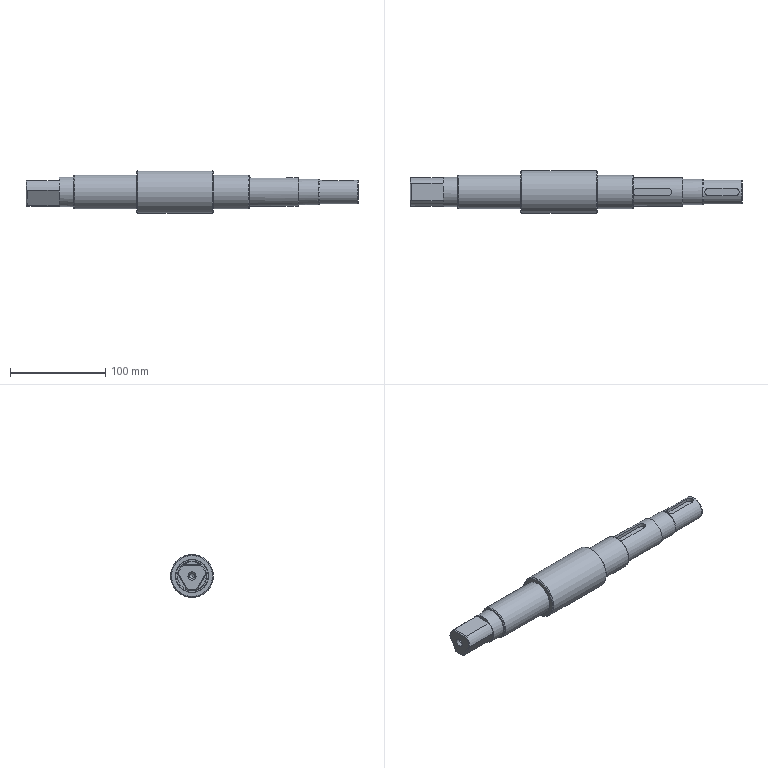NC program | NX | posted with a generic post | part box 348.4 x 45 x 45 mm
Lines 7257 to 8230 of 8230:
(PLANAR_MILL_COPY_COPY , TOOL : D6A45)
N14500 T07 M6
N14502 G54
N14504 G17 G0 G90 X13.51 Y-6.915 B0. C0. S7500 M3
N14506 G43 Z30. H7
N14508 Z0.5
N14510 G94 G1 Z-2.5 F1250.
N14512 G3 X12.818 Y-7.4 R1.
N14514 G1 X8.248 Y-15.315
N14516 G2 X6.473 Y-16.832 R3.5
N14518 X-6.473 Y-16.832 R18.034
N14520 X-8.248 Y-15.315 R3.5
N14522 G1 X-17.387 Y0.515
N14524 G2 X-17.813 Y2.81 R3.5
N14526 X-11.34 Y14.022 R18.034
N14528 X-9.139 Y14.801 R3.5
N14530 G1 X9.139
N14532 G2 X11.34 Y14.022 R3.5
N14534 X17.813 Y2.81 R18.034
N14536 X17.387 Y0.515 R3.5
N14538 G1 X12.818 Y-7.4
N14540 X12.385 Y-7.15
N14542 X7.815 Y-15.065
N14544 G2 X6.294 Y-16.365 R3.
N14546 X-6.294 Y-16.365 R17.534
N14548 X-7.815 Y-15.065 R3.
N14550 G1 X-16.954 Y0.765
N14552 G2 X-17.32 Y2.732 R3.
N14554 X-11.026 Y13.633 R17.534
N14556 X-9.139 Y14.301 R3.
N14558 G1 X9.139
N14560 G2 X11.026 Y13.633 R3.
N14562 X17.32 Y2.732 R17.534
N14564 X16.954 Y0.765 R3.
N14566 G1 X12.385 Y-7.15
N14568 X11.952 Y-6.9
N14570 X7.382 Y-14.815
N14572 G2 X6.114 Y-15.898 R2.5
N14574 X-6.114 Y-15.898 R17.034
N14576 X-7.382 Y-14.815 R2.5
N14578 G1 X-16.521 Y1.015
N14580 G2 X-16.826 Y2.654 R2.5
N14582 X-10.711 Y13.244 R17.034
N14584 X-9.139 Y13.801 R2.5
N14586 G1 X9.139
N14588 G2 X10.711 Y13.244 R2.5
N14590 X16.826 Y2.654 R17.034
N14592 X16.521 Y1.015 R2.5
N14594 G1 X11.952 Y-6.9
N14596 G3 X11.878 Y-7.742 R1.
N14598 G1 Z0.5
N14600 G0 Z30.
(PLANAR_MILL_COPY_COPY_COPY , TOOL : D6A45)
N14602 X0.766 Y1.143
N14604 Z1.5
N14606 G1 Z-1.5
N14608 G3 X0. Y1.5 R1.
N14610 X-1.5 Y0. R1.5
N14612 X0. Y1.5 R-1.5
N14614 X-0.766 Y1.143 R1.
N14616 G1 Z1.5
N14618 G0 Z30.
N14620 M5
(刀补12 , TOOL : D12)
N14622 T12 M6
N14624 G54
N14626 G17 G0 G90 X-12.039 Y-19.737 B0. C0. S5000 M3
N14628 G43 Z30. H12
N14630 Z1.
N14632 G94 G1 Z-1. F1250.
N14634 G41 X-11.975 Y-19.66 D12
N14636 X-11.079 Y-18.11
N14638 G3 X-11.079 Y-16.91 R1.2
N14640 G1 X-20.131 Y-1.232
N14642 G2 X-20.488 Y-0.507 R5.249
N14644 X-20.765 Y0.339 R6.776
N14646 X-20.863 Y2.801 R6.317
N14648 X-13.595 Y16.071 R21.05
N14650 X-12.592 Y16.868 R21.528
N14652 X-9.101 Y18.05 R6.061
N14654 G1 X-9.
N14656 X8.993
N14658 G2 X9.818 Y17.994 R5.44
N14660 X12.63 Y16.84 R6.029
N14662 X13.607 Y16.061 R21.048
N14664 X20.9 Y2.505 R21.
N14666 X20.133 Y-1.228 R6.039
N14668 G1 X11.132 Y-16.819
N14670 G2 X10.673 Y-17.502 R5.208
N14672 X8.257 Y-19.363 R6.188
N14674 X-8.171 Y-19.399 R21.05
N14676 X-11.079 Y-16.91 R6.067
N14678 G3 X-12.129 Y-16.329 R1.2
N14680 G1 X-14.165 Y-16.366
N14682 G40
N14684 X-14.263 Y-16.385
N14686 Z1.
N14688 G0 Z30.
N14690 X-12.002 Y-19.775
N14692 Z0.
N14694 G1 Z-2.
N14696 G41 X-11.939 Y-19.697
N14698 X-11.058 Y-18.109
N14700 G3 X-11.079 Y-16.909 R1.2
N14702 G1 X-11.132 Y-16.819
N14704 X-20.14 Y-1.217
N14706 G2 X-20.899 Y2.518 R6.05
N14708 X-12.63 Y16.84 R21.05
N14710 X-8.99 Y18.05 R6.05
N14712 G1 X9.
N14714 G2 X12.63 Y16.84 R6.05
N14716 X20.899 Y2.518 R21.05
N14718 X20.125 Y-1.243 R6.05
N14720 G1 X11.156 Y-16.777
N14722 X11.132 Y-16.82
N14724 G2 X8.269 Y-19.358 R6.05
N14726 X-8.269 Y-19.358 R21.05
N14728 X-11.079 Y-16.909 R6.05
N14730 G3 X-12.128 Y-16.327 R1.2
N14732 G1 X-14.167 Y-16.363
N14734 G40
N14736 X-14.265 Y-16.382
N14738 Z0.
N14740 G0 Z30.
N14742 X-12.002 Y-19.775
N14744 Z-1.
N14746 G1 Z-3.
N14748 G41 X-11.939 Y-19.697
N14750 X-11.058 Y-18.109
N14752 G3 X-11.079 Y-16.909 R1.2
N14754 G1 X-11.132 Y-16.819
N14756 X-20.14 Y-1.217
N14758 G2 X-20.899 Y2.518 R6.05
N14760 X-12.63 Y16.84 R21.05
N14762 X-8.99 Y18.05 R6.05
N14764 G1 X9.
N14766 G2 X12.63 Y16.84 R6.05
N14768 X20.899 Y2.518 R21.05
N14770 X20.125 Y-1.243 R6.05
N14772 G1 X11.156 Y-16.777
N14774 X11.131 Y-16.82
N14776 G2 X8.269 Y-19.358 R6.05
N14778 X-8.269 Y-19.358 R21.05
N14780 X-11.079 Y-16.909 R6.05
N14782 G3 X-12.128 Y-16.327 R1.2
N14784 G1 X-14.167 Y-16.363
N14786 G40
N14788 X-14.265 Y-16.382
N14790 Z-1.
N14792 G0 Z30.
N14794 X-12.002 Y-19.775
N14796 Z-2.
N14798 G1 Z-4.
N14800 G41 X-11.939 Y-19.697
N14802 X-11.058 Y-18.109
N14804 G3 X-11.079 Y-16.909 R1.2
N14806 G1 X-11.132 Y-16.819
N14808 X-20.14 Y-1.217
N14810 G2 X-20.899 Y2.518 R6.05
N14812 X-12.63 Y16.84 R21.05
N14814 X-8.99 Y18.05 R6.05
N14816 G1 X9.
N14818 G2 X12.63 Y16.84 R6.05
N14820 X20.899 Y2.518 R21.05
N14822 X20.125 Y-1.243 R6.05
N14824 G1 X11.156 Y-16.777
N14826 X11.131 Y-16.82
N14828 G2 X8.269 Y-19.358 R6.05
N14830 X-8.269 Y-19.358 R21.05
N14832 X-11.079 Y-16.909 R6.05
N14834 G3 X-12.128 Y-16.327 R1.2
N14836 G1 X-14.167 Y-16.363
N14838 G40
N14840 X-14.265 Y-16.382
N14842 Z-2.
N14844 G0 Z30.
N14846 X-12.002 Y-19.775
N14848 Z-3.
N14850 G1 Z-5.
N14852 G41 X-11.939 Y-19.697
N14854 X-11.058 Y-18.109
N14856 G3 X-11.079 Y-16.909 R1.2
N14858 G1 X-11.132 Y-16.819
N14860 X-20.14 Y-1.217
N14862 G2 X-20.899 Y2.518 R6.05
N14864 X-12.63 Y16.84 R21.05
N14866 X-8.99 Y18.05 R6.05
N14868 G1 X9.
N14870 G2 X12.63 Y16.84 R6.05
N14872 X20.899 Y2.518 R21.05
N14874 X20.125 Y-1.243 R6.05
N14876 G1 X11.156 Y-16.777
N14878 X11.131 Y-16.82
N14880 G2 X8.269 Y-19.358 R6.05
N14882 X-8.269 Y-19.358 R21.05
N14884 X-11.079 Y-16.909 R6.05
N14886 G3 X-12.128 Y-16.327 R1.2
N14888 G1 X-14.167 Y-16.363
N14890 G40
N14892 X-14.265 Y-16.382
N14894 Z-3.
N14896 G0 Z30.
N14898 X-12.002 Y-19.775
N14900 Z-4.
N14902 G1 Z-6.
N14904 G41 X-11.939 Y-19.697
N14906 X-11.058 Y-18.109
N14908 G3 X-11.079 Y-16.909 R1.2
N14910 G1 X-11.132 Y-16.819
N14912 X-20.14 Y-1.217
N14914 G2 X-20.899 Y2.518 R6.05
N14916 X-12.63 Y16.84 R21.05
N14918 X-8.99 Y18.05 R6.05
N14920 G1 X9.
N14922 G2 X12.63 Y16.84 R6.05
N14924 X20.899 Y2.518 R21.05
N14926 X20.125 Y-1.243 R6.05
N14928 G1 X11.156 Y-16.777
N14930 X11.131 Y-16.821
N14932 G2 X8.269 Y-19.358 R6.05
N14934 X-8.269 Y-19.358 R21.05
N14936 X-11.079 Y-16.909 R6.05
N14938 G3 X-12.128 Y-16.327 R1.2
N14940 G1 X-14.167 Y-16.363
N14942 G40
N14944 X-14.265 Y-16.382
N14946 Z-4.
N14948 G0 Z30.
N14950 X-12.002 Y-19.775
N14952 Z-5.
N14954 G1 Z-7.
N14956 G41 X-11.939 Y-19.697
N14958 X-11.058 Y-18.109
N14960 G3 X-11.079 Y-16.909 R1.2
N14962 G1 X-11.132 Y-16.819
N14964 X-20.14 Y-1.217
N14966 G2 X-20.899 Y2.518 R6.05
N14968 X-12.63 Y16.84 R21.05
N14970 X-8.99 Y18.05 R6.05
N14972 G1 X9.
N14974 G2 X12.63 Y16.84 R6.05
N14976 X20.899 Y2.518 R21.05
N14978 X20.125 Y-1.243 R6.05
N14980 G1 X11.156 Y-16.777
N14982 X11.131 Y-16.821
N14984 G2 X8.269 Y-19.358 R6.05
N14986 X-8.269 Y-19.358 R21.05
N14988 X-11.079 Y-16.909 R6.05
N14990 G3 X-12.128 Y-16.327 R1.2
N14992 G1 X-14.167 Y-16.363
N14994 G40
N14996 X-14.265 Y-16.382
N14998 Z-5.
N15000 G0 Z30.
N15002 X-12.002 Y-19.775
N15004 Z-6.
N15006 G1 Z-8.
N15008 G41 X-11.939 Y-19.697
N15010 X-11.058 Y-18.109
N15012 G3 X-11.079 Y-16.909 R1.2
N15014 G1 X-11.132 Y-16.819
N15016 X-20.132 Y-1.231
N15018 G2 X-20.899 Y2.518 R6.05
N15020 X-12.63 Y16.84 R21.05
N15022 X-8.99 Y18.05 R6.05
N15024 G1 X9.
N15026 G2 X12.63 Y16.84 R6.05
N15028 X20.899 Y2.518 R21.05
N15030 X20.125 Y-1.243 R6.05
N15032 G1 X11.156 Y-16.777
N15034 X11.131 Y-16.821
N15036 G2 X8.269 Y-19.358 R6.05
N15038 X-8.269 Y-19.358 R21.05
N15040 X-11.079 Y-16.909 R6.05
N15042 G3 X-12.128 Y-16.327 R1.2
N15044 G1 X-14.167 Y-16.363
N15046 G40
N15048 X-14.265 Y-16.382
N15050 Z-6.
N15052 G0 Z30.
N15054 X-12.002 Y-19.775
N15056 Z-7.
N15058 G1 Z-9.
N15060 G41 X-11.939 Y-19.697
N15062 X-11.058 Y-18.109
N15064 G3 X-11.079 Y-16.909 R1.2
N15066 G1 X-11.132 Y-16.819
N15068 X-20.132 Y-1.231
N15070 G2 X-20.899 Y2.518 R6.05
N15072 X-12.63 Y16.84 R21.05
N15074 X-8.99 Y18.05 R6.05
N15076 G1 X9.
N15078 G2 X12.63 Y16.84 R6.05
N15080 X20.899 Y2.518 R21.05
N15082 X20.125 Y-1.243 R6.05
N15084 G1 X11.156 Y-16.777
N15086 X11.13 Y-16.822
N15088 G2 X8.269 Y-19.358 R6.05
N15090 X-8.269 Y-19.358 R21.05
N15092 X-11.079 Y-16.909 R6.05
N15094 G3 X-12.128 Y-16.327 R1.2
N15096 G1 X-14.167 Y-16.363
N15098 G40
N15100 X-14.265 Y-16.382
N15102 Z-7.
N15104 G0 Z30.
N15106 X-12.002 Y-19.775
N15108 Z-8.
N15110 G1 Z-10.
N15112 G41 X-11.939 Y-19.697
N15114 X-11.058 Y-18.109
N15116 G3 X-11.079 Y-16.909 R1.2
N15118 G1 X-11.132 Y-16.819
N15120 X-20.132 Y-1.231
N15122 G2 X-20.899 Y2.518 R6.05
N15124 X-12.63 Y16.84 R21.05
N15126 X-8.99 Y18.05 R6.05
N15128 G1 X9.
N15130 G2 X12.63 Y16.84 R6.05
N15132 X20.899 Y2.518 R21.05
N15134 X20.125 Y-1.243 R6.05
N15136 G1 X11.156 Y-16.777
N15138 X11.13 Y-16.822
N15140 G2 X8.269 Y-19.358 R6.05
N15142 X-8.269 Y-19.358 R21.05
N15144 X-11.079 Y-16.909 R6.05
N15146 G3 X-12.128 Y-16.327 R1.2
N15148 G1 X-14.167 Y-16.363
N15150 G40
N15152 X-14.265 Y-16.382
N15154 Z-8.
N15156 G0 Z30.
N15158 X-12.002 Y-19.775
N15160 Z-9.
N15162 G1 Z-11.
N15164 G41 X-11.939 Y-19.697
N15166 X-11.058 Y-18.109
N15168 G3 X-11.079 Y-16.909 R1.2
N15170 G1 X-11.132 Y-16.819
N15172 X-20.132 Y-1.23
N15174 G2 X-20.899 Y2.518 R6.05
N15176 X-12.63 Y16.84 R21.05
N15178 X-8.99 Y18.05 R6.05
N15180 G1 X9.
N15182 G2 X12.63 Y16.84 R6.05
N15184 X20.899 Y2.518 R21.05
N15186 X20.125 Y-1.243 R6.05
N15188 G1 X11.156 Y-16.777
N15190 X11.13 Y-16.822
N15192 G2 X8.269 Y-19.358 R6.05
N15194 X-8.269 Y-19.358 R21.05
N15196 X-11.079 Y-16.909 R6.05
N15198 G3 X-12.128 Y-16.327 R1.2
N15200 G1 X-14.167 Y-16.363
N15202 G40
N15204 X-14.265 Y-16.382
N15206 Z-9.
N15208 G0 Z30.
N15210 X-12.002 Y-19.775
N15212 Z-10.
N15214 G1 Z-12.
N15216 G41 X-11.939 Y-19.697
N15218 X-11.058 Y-18.109
N15220 G3 X-11.079 Y-16.909 R1.2
N15222 G1 X-11.132 Y-16.819
N15224 X-20.132 Y-1.23
N15226 G2 X-20.899 Y2.518 R6.05
N15228 X-12.63 Y16.84 R21.05
N15230 X-8.99 Y18.05 R6.05
N15232 G1 X9.
N15234 G2 X12.63 Y16.84 R6.05
N15236 X20.899 Y2.518 R21.05
N15238 X20.125 Y-1.243 R6.05
N15240 G1 X11.156 Y-16.777
N15242 X11.13 Y-16.823
N15244 G2 X8.269 Y-19.358 R6.05
N15246 X-8.269 Y-19.358 R21.05
N15248 X-11.079 Y-16.909 R6.05
N15250 G3 X-12.128 Y-16.327 R1.2
N15252 G1 X-14.167 Y-16.363
N15254 G40
N15256 X-14.265 Y-16.382
N15258 Z-10.
N15260 G0 Z30.
N15262 X-12.002 Y-19.775
N15264 Z-11.
N15266 G1 Z-13.
N15268 G41 X-11.939 Y-19.697
N15270 X-11.058 Y-18.109
N15272 G3 X-11.079 Y-16.909 R1.2
N15274 G1 X-11.132 Y-16.819
N15276 X-20.132 Y-1.23
N15278 G2 X-20.899 Y2.518 R6.05
N15280 X-12.63 Y16.84 R21.05
N15282 X-8.99 Y18.05 R6.05
N15284 G1 X9.
N15286 G2 X12.63 Y16.84 R6.05
N15288 X20.899 Y2.518 R21.05
N15290 X20.125 Y-1.243 R6.05
N15292 G1 X11.156 Y-16.777
N15294 X11.129 Y-16.823
N15296 G2 X8.269 Y-19.358 R6.05
N15298 X-8.269 Y-19.358 R21.05
N15300 X-11.079 Y-16.909 R6.05
N15302 G3 X-12.128 Y-16.327 R1.2
N15304 G1 X-14.167 Y-16.363
N15306 G40
N15308 X-14.265 Y-16.382
N15310 Z-11.
N15312 G0 Z30.
N15314 X-12.002 Y-19.775
N15316 Z-12.
N15318 G1 Z-14.
N15320 G41 X-11.939 Y-19.697
N15322 X-11.058 Y-18.109
N15324 G3 X-11.079 Y-16.909 R1.2
N15326 G1 X-11.132 Y-16.819
N15328 X-20.133 Y-1.229
N15330 G2 X-20.899 Y2.518 R6.05
N15332 X-12.63 Y16.84 R21.05
N15334 X-8.99 Y18.05 R6.05
N15336 G1 X9.
N15338 G2 X12.63 Y16.84 R6.05
N15340 X20.899 Y2.518 R21.05
N15342 X20.125 Y-1.243 R6.05
N15344 G1 X11.156 Y-16.777
N15346 X11.129 Y-16.824
N15348 G2 X8.269 Y-19.358 R6.05
N15350 X-8.269 Y-19.358 R21.05
N15352 X-11.079 Y-16.909 R6.05
N15354 G3 X-12.128 Y-16.327 R1.2
N15356 G1 X-14.167 Y-16.363
N15358 G40
N15360 X-14.265 Y-16.382
N15362 Z-12.
N15364 G0 Z30.
N15366 X-12.002 Y-19.775
N15368 Z-13.
N15370 G1 Z-15.
N15372 G41 X-11.939 Y-19.697
N15374 X-11.058 Y-18.109
N15376 G3 X-11.079 Y-16.909 R1.2
N15378 G1 X-11.132 Y-16.819
N15380 X-20.133 Y-1.229
N15382 G2 X-20.899 Y2.518 R6.05
N15384 X-12.63 Y16.84 R21.05
N15386 X-8.99 Y18.05 R6.05
N15388 G1 X9.
N15390 G2 X12.63 Y16.84 R6.05
N15392 X20.899 Y2.518 R21.05
N15394 X20.125 Y-1.243 R6.05
N15396 G1 X11.156 Y-16.777
N15398 X11.129 Y-16.824
N15400 G2 X8.269 Y-19.358 R6.05
N15402 X-8.269 Y-19.358 R21.05
N15404 X-11.079 Y-16.909 R6.05
N15406 G3 X-12.128 Y-16.327 R1.2
N15408 G1 X-14.167 Y-16.363
N15410 G40
N15412 X-14.265 Y-16.382
N15414 Z-13.
N15416 G0 Z30.
N15418 X-12.002 Y-19.775
N15420 Z-14.
N15422 G1 Z-16.
N15424 G41 X-11.939 Y-19.697
N15426 X-11.058 Y-18.109
N15428 G3 X-11.079 Y-16.909 R1.2
N15430 G1 X-11.132 Y-16.819
N15432 X-20.133 Y-1.229
N15434 G2 X-20.899 Y2.518 R6.05
N15436 X-12.63 Y16.84 R21.05
N15438 X-8.99 Y18.05 R6.05
N15440 G1 X9.
N15442 G2 X12.63 Y16.84 R6.05
N15444 X20.899 Y2.518 R21.05
N15446 X20.125 Y-1.243 R6.05
N15448 G1 X11.156 Y-16.777
N15450 X11.129 Y-16.825
N15452 G2 X8.269 Y-19.358 R6.05
N15454 X-8.269 Y-19.358 R21.05
N15456 X-11.079 Y-16.909 R6.05
N15458 G3 X-12.128 Y-16.327 R1.2
N15460 G1 X-14.167 Y-16.363
N15462 G40
N15464 X-14.265 Y-16.382
N15466 Z-14.
N15468 G0 Z30.
N15470 X-12.002 Y-19.775
N15472 Z-15.
N15474 G1 Z-17.
N15476 G41 X-11.939 Y-19.697
N15478 X-11.058 Y-18.109
N15480 G3 X-11.079 Y-16.909 R1.2
N15482 G1 X-11.132 Y-16.819
N15484 X-20.133 Y-1.228
N15486 G2 X-20.899 Y2.518 R6.05
N15488 X-12.63 Y16.84 R21.05
N15490 X-8.99 Y18.05 R6.05
N15492 G1 X9.
N15494 G2 X12.63 Y16.84 R6.05
N15496 X20.899 Y2.518 R21.05
N15498 X20.125 Y-1.243 R6.05
N15500 G1 X11.156 Y-16.777
N15502 X11.128 Y-16.825
N15504 G2 X8.269 Y-19.358 R6.05
N15506 X-8.269 Y-19.358 R21.05
N15508 X-11.079 Y-16.909 R6.05
N15510 G3 X-12.128 Y-16.327 R1.2
N15512 G1 X-14.167 Y-16.363
N15514 G40
N15516 X-14.265 Y-16.382
N15518 Z-15.
N15520 G0 Z30.
N15522 X-12.002 Y-19.775
N15524 Z-16.
N15526 G1 Z-18.
N15528 G41 X-11.939 Y-19.697
N15530 X-11.058 Y-18.109
N15532 G3 X-11.079 Y-16.909 R1.2
N15534 G1 X-11.132 Y-16.819
N15536 X-20.134 Y-1.227
N15538 G2 X-20.899 Y2.518 R6.05
N15540 X-12.63 Y16.84 R21.05
N15542 X-8.99 Y18.05 R6.05
N15544 G1 X9.
N15546 G2 X12.63 Y16.84 R6.05
N15548 X20.899 Y2.518 R21.05
N15550 X20.125 Y-1.243 R6.05
N15552 G1 X11.156 Y-16.777
N15554 X11.128 Y-16.826
N15556 G2 X8.269 Y-19.358 R6.05
N15558 X-8.269 Y-19.358 R21.05
N15560 X-11.079 Y-16.909 R6.05
N15562 G3 X-12.128 Y-16.327 R1.2
N15564 G1 X-14.167 Y-16.363
N15566 G40
N15568 X-14.265 Y-16.382
N15570 Z-16.
N15572 G0 Z30.
N15574 X-12.002 Y-19.775
N15576 Z-17.
N15578 G1 Z-19.
N15580 G41 X-11.939 Y-19.697
N15582 X-11.058 Y-18.109
N15584 G3 X-11.079 Y-16.909 R1.2
N15586 G1 X-11.132 Y-16.819
N15588 X-20.134 Y-1.227
N15590 G2 X-20.899 Y2.518 R6.05
N15592 X-12.63 Y16.84 R21.05
N15594 X-8.99 Y18.05 R6.05
N15596 G1 X9.
N15598 G2 X12.63 Y16.84 R6.05
N15600 X20.899 Y2.518 R21.05
N15602 X20.132 Y-1.231 R6.05
N15604 G1 X11.156 Y-16.777
N15606 X11.127 Y-16.827
N15608 G2 X8.269 Y-19.358 R6.05
N15610 X-8.269 Y-19.358 R21.05
N15612 X-11.079 Y-16.909 R6.05
N15614 G3 X-12.128 Y-16.327 R1.2
N15616 G1 X-14.167 Y-16.363
N15618 G40
N15620 X-14.265 Y-16.382
N15622 Z-17.
N15624 G0 Z30.
N15626 X-12.002 Y-19.775
N15628 Z-18.
N15630 G1 Z-20.
N15632 G41 X-11.939 Y-19.697
N15634 X-11.058 Y-18.109
N15636 G3 X-11.079 Y-16.909 R1.2
N15638 G1 X-11.132 Y-16.819
N15640 X-20.134 Y-1.226
N15642 G2 X-20.899 Y2.518 R6.05
N15644 X-12.63 Y16.84 R21.05
N15646 X-8.99 Y18.05 R6.05
N15648 G1 X9.
N15650 G2 X12.63 Y16.84 R6.05
N15652 X20.899 Y2.518 R21.05
N15654 X20.132 Y-1.231 R6.05
N15656 G1 X11.132 Y-16.819
N15658 G2 X8.269 Y-19.358 R6.05
N15660 X-8.269 Y-19.358 R21.05
N15662 X-11.079 Y-16.909 R6.05
N15664 G3 X-12.128 Y-16.327 R1.2
N15666 G1 X-14.167 Y-16.363
N15668 G40
N15670 X-14.265 Y-16.382
N15672 Z-18.
N15674 G0 Z30.
N15676 X-12.002 Y-19.775
N15678 Z-19.
N15680 G1 Z-21.
N15682 G41 X-11.939 Y-19.697
N15684 X-11.058 Y-18.109
N15686 G3 X-11.079 Y-16.909 R1.2
N15688 G1 X-11.132 Y-16.819
N15690 X-20.135 Y-1.225
N15692 G2 X-20.899 Y2.518 R6.05
N15694 X-12.63 Y16.84 R21.05
N15696 X-9. Y18.05 R6.05
N15698 G1 X9.
N15700 G2 X12.63 Y16.84 R6.05
N15702 X20.899 Y2.518 R21.05
N15704 X20.132 Y-1.231 R6.05
N15706 G1 X11.132 Y-16.819
N15708 G2 X8.269 Y-19.358 R6.05
N15710 X-8.269 Y-19.358 R21.05
N15712 X-11.079 Y-16.909 R6.05
N15714 G3 X-12.128 Y-16.327 R1.2
N15716 G1 X-14.167 Y-16.363
N15718 G40
N15720 X-14.265 Y-16.382
N15722 Z-19.
N15724 G0 Z30.
N15726 X-12.002 Y-19.775
N15728 Z-20.
N15730 G1 Z-22.
N15732 G41 X-11.939 Y-19.697
N15734 X-11.058 Y-18.109
N15736 G3 X-11.079 Y-16.909 R1.2
N15738 G1 X-11.132 Y-16.819
N15740 X-20.135 Y-1.224
N15742 G2 X-20.899 Y2.518 R6.05
N15744 X-12.63 Y16.84 R21.05
N15746 X-9. Y18.05 R6.05
N15748 G1 X9.
N15750 G2 X12.63 Y16.84 R6.05
N15752 X20.899 Y2.518 R21.05
N15754 X20.132 Y-1.231 R6.05
N15756 G1 X11.132 Y-16.819
N15758 G2 X8.269 Y-19.358 R6.05
N15760 X-8.269 Y-19.358 R21.05
N15762 X-11.079 Y-16.909 R6.05
N15764 G3 X-12.128 Y-16.327 R1.2
N15766 G1 X-14.167 Y-16.363
N15768 G40
N15770 X-14.265 Y-16.382
N15772 Z-20.
N15774 G0 Z30.
N15776 X-12.002 Y-19.775
N15778 Z-21.
N15780 G1 Z-23.
N15782 G41 X-11.939 Y-19.697
N15784 X-11.058 Y-18.109
N15786 G3 X-11.079 Y-16.909 R1.2
N15788 G1 X-11.132 Y-16.819
N15790 X-20.136 Y-1.223
N15792 G2 X-20.899 Y2.518 R6.05
N15794 X-12.63 Y16.84 R21.05
N15796 X-9. Y18.05 R6.05
N15798 G1 X9.
N15800 G2 X12.63 Y16.84 R6.05
N15802 X20.899 Y2.518 R21.05
N15804 X20.132 Y-1.231 R6.05
N15806 G1 X11.132 Y-16.819
N15808 G2 X8.269 Y-19.358 R6.05
N15810 X-8.269 Y-19.358 R21.05
N15812 X-11.079 Y-16.909 R6.05
N15814 G3 X-12.128 Y-16.327 R1.2
N15816 G1 X-14.167 Y-16.363
N15818 G40
N15820 X-14.265 Y-16.382
N15822 Z-21.
N15824 G0 Z30.
N15826 X-12.002 Y-19.775
N15828 Z-22.
N15830 G1 Z-24.
N15832 G41 X-11.939 Y-19.697
N15834 X-11.058 Y-18.109
N15836 G3 X-11.079 Y-16.909 R1.2
N15838 G1 X-11.132 Y-16.819
N15840 X-20.132 Y-1.231
N15842 G2 X-20.899 Y2.518 R6.05
N15844 X-12.63 Y16.84 R21.05
N15846 X-9. Y18.05 R6.05
N15848 G1 X9.
N15850 G2 X12.63 Y16.84 R6.05
N15852 X20.899 Y2.518 R21.05
N15854 X20.132 Y-1.231 R6.05
N15856 G1 X11.132 Y-16.819
N15858 G2 X8.269 Y-19.358 R6.05
N15860 X-8.269 Y-19.358 R21.05
N15862 X-11.079 Y-16.909 R6.05
N15864 G3 X-12.128 Y-16.327 R1.2
N15866 G1 X-14.167 Y-16.363
N15868 G40
N15870 X-14.265 Y-16.382
N15872 Z-22.
N15874 G0 Z30.
N15876 X-12.002 Y-19.775
N15878 Z-23.
N15880 G1 Z-25.
N15882 G41 X-11.939 Y-19.697
N15884 X-11.058 Y-18.109
N15886 G3 X-11.079 Y-16.909 R1.2
N15888 G1 X-11.132 Y-16.819
N15890 X-20.132 Y-1.231
N15892 G2 X-20.899 Y2.518 R6.05
N15894 X-12.63 Y16.84 R21.05
N15896 X-9. Y18.05 R6.05
N15898 G1 X9.
N15900 G2 X12.63 Y16.84 R6.05
N15902 X20.899 Y2.518 R21.05
N15904 X20.132 Y-1.231 R6.05
N15906 G1 X11.132 Y-16.819
N15908 G2 X8.269 Y-19.358 R6.05
N15910 X-8.269 Y-19.358 R21.05
N15912 X-11.079 Y-16.909 R6.05
N15914 G3 X-12.128 Y-16.327 R1.2
N15916 G1 X-14.167 Y-16.363
N15918 G40
N15920 X-14.265 Y-16.382
N15922 Z-23.
N15924 G0 Z30.
N15926 X-12.002 Y-19.775
N15928 Z-24.
N15930 G1 Z-26.
N15932 G41 X-11.939 Y-19.697
N15934 X-11.058 Y-18.109
N15936 G3 X-11.079 Y-16.909 R1.2
N15938 G1 X-11.132 Y-16.819
N15940 X-20.132 Y-1.231
N15942 G2 X-20.899 Y2.518 R6.05
N15944 X-12.63 Y16.84 R21.05
N15946 X-9. Y18.05 R6.05
N15948 G1 X9.
N15950 G2 X12.63 Y16.84 R6.05
N15952 X20.899 Y2.518 R21.05
N15954 X20.132 Y-1.231 R6.05
N15956 G1 X11.132 Y-16.819
N15958 G2 X8.269 Y-19.358 R6.05
N15960 X-8.269 Y-19.358 R21.05
N15962 X-11.079 Y-16.909 R6.05
N15964 G3 X-12.128 Y-16.327 R1.2
N15966 G1 X-14.167 Y-16.363
N15968 G40
N15970 X-14.265 Y-16.382
N15972 Z-24.
N15974 G0 Z30.
N15976 X-12.002 Y-19.775
N15978 Z-25.
N15980 G1 Z-27.
N15982 G41 X-11.939 Y-19.697
N15984 X-11.058 Y-18.109
N15986 G3 X-11.079 Y-16.909 R1.2
N15988 G1 X-11.132 Y-16.819
N15990 X-20.132 Y-1.231
N15992 G2 X-20.899 Y2.518 R6.05
N15994 X-12.63 Y16.84 R21.05
N15996 X-9. Y18.05 R6.05
N15998 G1 X9.
N16000 G2 X12.63 Y16.84 R6.05
N16002 X20.899 Y2.518 R21.05
N16004 X20.132 Y-1.231 R6.05
N16006 G1 X11.132 Y-16.819
N16008 G2 X8.269 Y-19.358 R6.05
N16010 X-8.269 Y-19.358 R21.05
N16012 X-11.079 Y-16.909 R6.05
N16014 G3 X-12.128 Y-16.327 R1.2
N16016 G1 X-14.167 Y-16.363
N16018 G40
N16020 X-14.265 Y-16.382
N16022 Z-25.
N16024 G0 Z30.
N16026 X-12.002 Y-19.775
N16028 Z-26.
N16030 G1 Z-28.
N16032 G41 X-11.939 Y-19.697
N16034 X-11.058 Y-18.109
N16036 G3 X-11.079 Y-16.909 R1.2
N16038 G1 X-11.132 Y-16.819
N16040 X-20.132 Y-1.231
N16042 G2 X-20.899 Y2.518 R6.05
N16044 X-12.63 Y16.84 R21.05
N16046 X-9. Y18.05 R6.05
N16048 G1 X9.
N16050 G2 X12.63 Y16.84 R6.05
N16052 X20.899 Y2.518 R21.05
N16054 X20.132 Y-1.231 R6.05
N16056 G1 X11.132 Y-16.819
N16058 G2 X8.269 Y-19.358 R6.05
N16060 X-8.269 Y-19.358 R21.05
N16062 X-11.079 Y-16.909 R6.05
N16064 G3 X-12.128 Y-16.327 R1.2
N16066 G1 X-14.167 Y-16.363
N16068 G40
N16070 X-14.265 Y-16.382
N16072 Z-26.
N16074 G0 Z30.
N16076 X-12.002 Y-19.775
N16078 Z-27.
N16080 G1 Z-29.
N16082 G41 X-11.939 Y-19.697
N16084 X-11.058 Y-18.109
N16086 G3 X-11.079 Y-16.909 R1.2
N16088 G1 X-11.132 Y-16.819
N16090 X-20.132 Y-1.231
N16092 G2 X-20.899 Y2.518 R6.05
N16094 X-12.63 Y16.84 R21.05
N16096 X-9. Y18.05 R6.05
N16098 G1 X9.
N16100 G2 X12.63 Y16.84 R6.05
N16102 X20.899 Y2.518 R21.05
N16104 X20.132 Y-1.231 R6.05
N16106 G1 X11.132 Y-16.819
N16108 G2 X8.269 Y-19.358 R6.05
N16110 X-8.269 Y-19.358 R21.05
N16112 X-11.079 Y-16.909 R6.05
N16114 G3 X-12.128 Y-16.327 R1.2
N16116 G1 X-14.167 Y-16.363
N16118 G40
N16120 X-14.265 Y-16.382
N16122 Z-27.
N16124 G0 Z30.
N16126 X-12.002 Y-19.775
N16128 Z-28.
N16130 G1 Z-30.
N16132 G41 X-11.939 Y-19.697
N16134 X-11.058 Y-18.109
N16136 G3 X-11.079 Y-16.909 R1.2
N16138 G1 X-11.132 Y-16.819
N16140 X-20.132 Y-1.231
N16142 G2 X-20.899 Y2.518 R6.05
N16144 X-12.63 Y16.84 R21.05
N16146 X-9. Y18.05 R6.05
N16148 G1 X9.
N16150 G2 X12.63 Y16.84 R6.05
N16152 X20.899 Y2.518 R21.05
N16154 X20.132 Y-1.231 R6.05
N16156 G1 X11.132 Y-16.819
N16158 G2 X8.269 Y-19.358 R6.05
N16160 X-8.269 Y-19.358 R21.05
N16162 X-11.079 Y-16.909 R6.05
N16164 G3 X-12.128 Y-16.327 R1.2
N16166 G1 X-14.167 Y-16.363
N16168 G40
N16170 X-14.265 Y-16.382
N16172 Z-28.
N16174 G0 Z30.
N16176 X-12.002 Y-19.775
N16178 Z-29.
N16180 G1 Z-31.
N16182 G41 X-11.939 Y-19.697
N16184 X-11.058 Y-18.109
N16186 G3 X-11.079 Y-16.909 R1.2
N16188 G1 X-11.132 Y-16.819
N16190 X-20.132 Y-1.231
N16192 G2 X-20.899 Y2.518 R6.05
N16194 X-12.63 Y16.84 R21.05
N16196 X-9. Y18.05 R6.05
N16198 G1 X9.
N16200 G2 X12.63 Y16.84 R6.05
N16202 X20.899 Y2.518 R21.05
N16204 X20.132 Y-1.231 R6.05
N16206 G1 X11.132 Y-16.819
N16208 G2 X8.269 Y-19.358 R6.05
N16210 X-8.269 Y-19.358 R21.05
N16212 X-11.079 Y-16.909 R6.05
N16214 G3 X-12.128 Y-16.327 R1.2
N16216 G1 X-14.167 Y-16.363
N16218 G40
N16220 X-14.265 Y-16.382
N16222 Z-29.
N16224 G0 Z30.
N16226 X-12.002 Y-19.775
N16228 Z-30.
N16230 G1 Z-32.
N16232 G41 X-11.939 Y-19.697
N16234 X-11.058 Y-18.109
N16236 G3 X-11.079 Y-16.909 R1.2
N16238 G1 X-11.132 Y-16.819
N16240 X-20.132 Y-1.231
N16242 G2 X-20.899 Y2.518 R6.05
N16244 X-12.63 Y16.84 R21.05
N16246 X-9. Y18.05 R6.05
N16248 G1 X9.
N16250 G2 X12.63 Y16.84 R6.05
N16252 X20.899 Y2.518 R21.05
N16254 X20.132 Y-1.231 R6.05
N16256 G1 X11.132 Y-16.819
N16258 G2 X8.269 Y-19.358 R6.05
N16260 X-8.269 Y-19.358 R21.05
N16262 X-11.079 Y-16.909 R6.05
N16264 G3 X-12.128 Y-16.327 R1.2
N16266 G1 X-14.167 Y-16.363
N16268 G40
N16270 X-14.265 Y-16.382
N16272 Z-30.
N16274 G0 Z30.
N16276 X-12.002 Y-19.775
N16278 Z-31.
N16280 G1 Z-33.
N16282 G41 X-11.939 Y-19.697
N16284 X-11.058 Y-18.109
N16286 G3 X-11.079 Y-16.909 R1.2
N16288 G1 X-11.132 Y-16.819
N16290 X-20.132 Y-1.231
N16292 G2 X-20.899 Y2.518 R6.05
N16294 X-12.63 Y16.84 R21.05
N16296 X-9. Y18.05 R6.05
N16298 G1 X9.
N16300 G2 X12.63 Y16.84 R6.05
N16302 X20.899 Y2.518 R21.05
N16304 X20.132 Y-1.231 R6.05
N16306 G1 X11.132 Y-16.819
N16308 G2 X8.269 Y-19.358 R6.05
N16310 X-8.269 Y-19.358 R21.05
N16312 X-11.079 Y-16.909 R6.05
N16314 G3 X-12.128 Y-16.327 R1.2
N16316 G1 X-14.167 Y-16.363
N16318 G40
N16320 X-14.265 Y-16.382
N16322 Z-31.
N16324 G0 Z30.
N16326 X-12.002 Y-19.775
N16328 Z-32.
N16330 G1 Z-34.
N16332 G41 X-11.939 Y-19.697
N16334 X-11.058 Y-18.109
N16336 G3 X-11.079 Y-16.909 R1.2
N16338 G1 X-11.132 Y-16.819
N16340 X-20.132 Y-1.231
N16342 G2 X-20.899 Y2.518 R6.05
N16344 X-12.63 Y16.84 R21.05
N16346 X-9. Y18.05 R6.05
N16348 G1 X9.
N16350 G2 X12.63 Y16.84 R6.05
N16352 X20.899 Y2.518 R21.05
N16354 X20.132 Y-1.231 R6.05
N16356 G1 X11.132 Y-16.819
N16358 G2 X8.269 Y-19.358 R6.05
N16360 X-8.269 Y-19.358 R21.05
N16362 X-11.079 Y-16.909 R6.05
N16364 G3 X-12.128 Y-16.327 R1.2
N16366 G1 X-14.167 Y-16.363
N16368 G40
N16370 X-14.265 Y-16.382
N16372 Z-32.
N16374 G0 Z30.
N16376 X-12.002 Y-19.775
N16378 Z-33.
N16380 G1 Z-35.
N16382 G41 X-11.939 Y-19.697
N16384 X-11.058 Y-18.109
N16386 G3 X-11.079 Y-16.909 R1.2
N16388 G1 X-11.132 Y-16.819
N16390 X-20.132 Y-1.231
N16392 G2 X-20.899 Y2.518 R6.05
N16394 X-12.63 Y16.84 R21.05
N16396 X-9. Y18.05 R6.05
N16398 G1 X9.
N16400 G2 X12.63 Y16.84 R6.05
N16402 X20.899 Y2.518 R21.05
N16404 X20.132 Y-1.231 R6.05
N16406 G1 X11.132 Y-16.819
N16408 G2 X8.269 Y-19.358 R6.05
N16410 X-8.269 Y-19.358 R21.05
N16412 X-11.079 Y-16.909 R6.05
N16414 G3 X-12.128 Y-16.327 R1.2
N16416 G1 X-14.167 Y-16.363
N16418 G40
N16420 X-14.265 Y-16.382
N16422 Z-33.
N16424 G0 Z30.
N16426 M5
N16428 M2